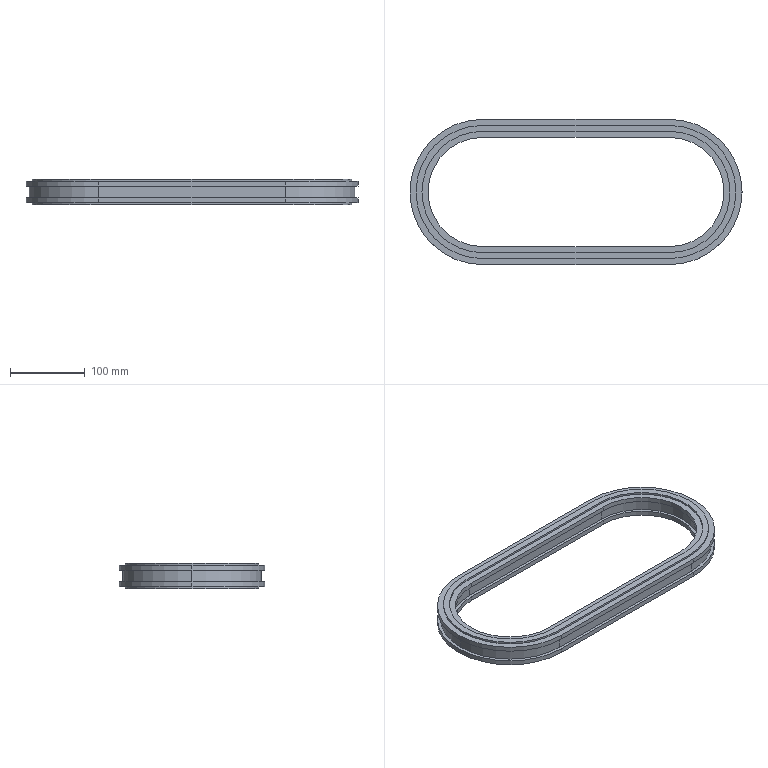Part | SolidWorks | 1 solid | 60 faces | box 444.526 x 194.526 x 33.528 mm | volume 618540 mm3 | cylinder 30 | plane 30 | commonest cylinder face diameters 146.317 x6 162.497 x6 178.346 x6 194.526 x6 154.546 x3 186.296 x3